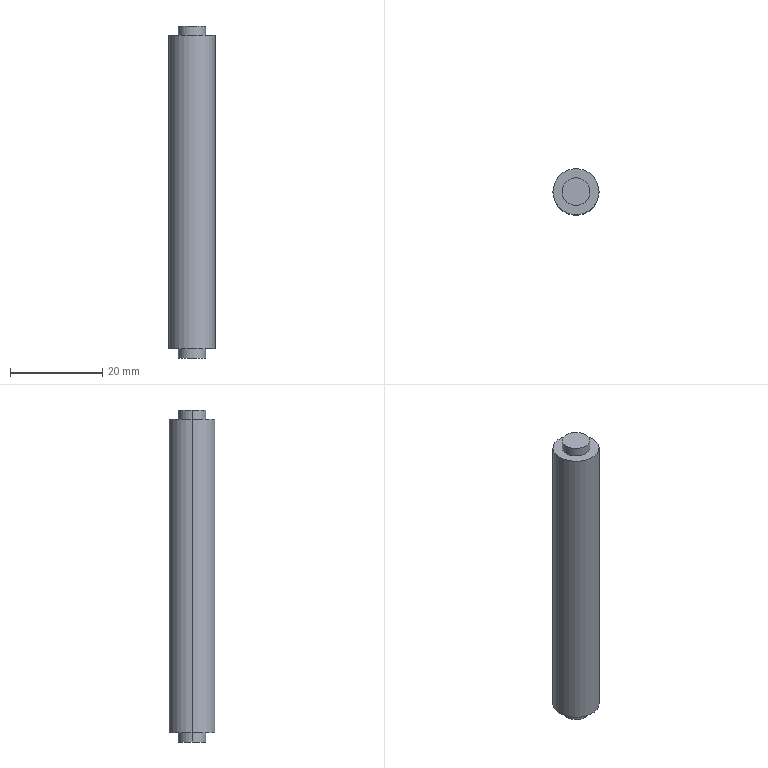Part | STEP file | 1 solid | 10 faces | box 10 x 10 x 72 mm | volume 5454 mm3 | cylinder 6 | plane 4 | commonest cylinder face diameters 6 x4 10 x2
STEP:
#1=CARTESIAN_POINT('',(0.,0.,0.));
#2=DIRECTION('',(0.,0.,1.));
#3=DIRECTION('',(1.,0.,0.));
#4=AXIS2_PLACEMENT_3D('',#1,#2,#3);
#5=CARTESIAN_POINT('',(182.13,-201.166,-34.));
#6=VERTEX_POINT('',#5);
#7=CARTESIAN_POINT('',(172.13,-201.166,-34.));
#8=VERTEX_POINT('',#7);
#9=CARTESIAN_POINT('',(177.13,-201.166,-34.));
#10=DIRECTION('',(0.,0.,1.));
#11=DIRECTION('',(1.,0.,0.));
#12=AXIS2_PLACEMENT_3D('',#9,#10,#11);
#13=CIRCLE('',#12,5.);
#14=CARTESIAN_POINT('',(177.13,-201.166,0.));
#15=DIRECTION('',(0.,0.,1.));
#16=DIRECTION('',(1.,0.,0.));
#17=AXIS2_PLACEMENT_3D('',#14,#15,#16);
#18=CYLINDRICAL_SURFACE('',#17,5.);
#19=CARTESIAN_POINT('',(0.,-34.));
#20=DIRECTION('',(1.,0.));
#21=VECTOR('',#20,1.);
#22=LINE('',#19,#21);
#23=(GEOMETRIC_REPRESENTATION_CONTEXT(2)PARAMETRIC_REPRESENTATION_CONTEXT()REPRESENTATION_CONTEXT('',''));
#24=DEFINITIONAL_REPRESENTATION('',(#22),#23);
#25=PCURVE('',#18,#24);
#26=CARTESIAN_POINT('',(177.13,-201.166,-34.));
#27=DIRECTION('',(0.,0.,1.));
#28=DIRECTION('',(1.,0.,0.));
#29=AXIS2_PLACEMENT_3D('',#26,#27,#28);
#30=PLANE('',#29);
#31=CARTESIAN_POINT('',(0.,0.));
#32=DIRECTION('',(1.,0.));
#33=AXIS2_PLACEMENT_2D('',#31,#32);
#34=CIRCLE('',#33,5.);
#35=(GEOMETRIC_REPRESENTATION_CONTEXT(2)PARAMETRIC_REPRESENTATION_CONTEXT()REPRESENTATION_CONTEXT('',''));
#36=DEFINITIONAL_REPRESENTATION('',(#34),#35);
#37=PCURVE('',#30,#36);
#38=SURFACE_CURVE('',#13,(#25,#37),.PCURVE_S1.);
#39=EDGE_CURVE('',#6,#8,#38,.T.);
#40=ORIENTED_EDGE('',*,*,#39,.T.);
#41=CARTESIAN_POINT('',(172.13,-201.166,34.));
#42=VERTEX_POINT('',#41);
#43=CARTESIAN_POINT('',(172.13,-201.166,0.));
#44=DIRECTION('',(0.,0.,1.));
#45=VECTOR('',#44,1.);
#46=LINE('',#43,#45);
#47=CARTESIAN_POINT('',(3.142,0.));
#48=DIRECTION('',(0.,1.));
#49=VECTOR('',#48,1.);
#50=LINE('',#47,#49);
#51=(GEOMETRIC_REPRESENTATION_CONTEXT(2)PARAMETRIC_REPRESENTATION_CONTEXT()REPRESENTATION_CONTEXT('',''));
#52=DEFINITIONAL_REPRESENTATION('',(#50),#51);
#53=PCURVE('',#18,#52);
#54=CARTESIAN_POINT('',(177.13,-201.166,0.));
#55=DIRECTION('',(0.,0.,1.));
#56=DIRECTION('',(1.,0.,0.));
#57=AXIS2_PLACEMENT_3D('',#54,#55,#56);
#58=CYLINDRICAL_SURFACE('',#57,5.);
#59=CARTESIAN_POINT('',(3.142,0.));
#60=DIRECTION('',(0.,1.));
#61=VECTOR('',#60,1.);
#62=LINE('',#59,#61);
#63=(GEOMETRIC_REPRESENTATION_CONTEXT(2)PARAMETRIC_REPRESENTATION_CONTEXT()REPRESENTATION_CONTEXT('',''));
#64=DEFINITIONAL_REPRESENTATION('',(#62),#63);
#65=PCURVE('',#58,#64);
#66=SURFACE_CURVE('',#46,(#53,#65),.PCURVE_S1.);
#67=EDGE_CURVE('',#8,#42,#66,.T.);
#68=ORIENTED_EDGE('',*,*,#67,.T.);
#69=CARTESIAN_POINT('',(182.13,-201.166,34.));
#70=VERTEX_POINT('',#69);
#71=CARTESIAN_POINT('',(177.13,-201.166,34.));
#72=DIRECTION('',(0.,0.,-1.));
#73=DIRECTION('',(1.,0.,0.));
#74=AXIS2_PLACEMENT_3D('',#71,#72,#73);
#75=CIRCLE('',#74,5.);
#76=CARTESIAN_POINT('',(6.283,34.));
#77=DIRECTION('',(-1.,0.));
#78=VECTOR('',#77,1.);
#79=LINE('',#76,#78);
#80=(GEOMETRIC_REPRESENTATION_CONTEXT(2)PARAMETRIC_REPRESENTATION_CONTEXT()REPRESENTATION_CONTEXT('',''));
#81=DEFINITIONAL_REPRESENTATION('',(#79),#80);
#82=PCURVE('',#18,#81);
#83=CARTESIAN_POINT('',(177.13,-201.166,34.));
#84=DIRECTION('',(0.,0.,1.));
#85=DIRECTION('',(1.,0.,0.));
#86=AXIS2_PLACEMENT_3D('',#83,#84,#85);
#87=PLANE('',#86);
#88=CARTESIAN_POINT('',(5.,0.));
#89=CARTESIAN_POINT('',(5.,-8.66));
#90=CARTESIAN_POINT('',(-2.5,-4.33));
#91=CARTESIAN_POINT('',(-10.,0.));
#92=CARTESIAN_POINT('',(-2.5,4.33));
#93=CARTESIAN_POINT('',(5.,8.66));
#94=CARTESIAN_POINT('',(5.,0.));
#95=(BOUNDED_CURVE()B_SPLINE_CURVE(2,(#88,#89,#90,#91,#92,#93,#94),.UNSPECIFIED.,.T.,.F.)B_SPLINE_CURVE_WITH_KNOTS((1,2,2,2,2,1),(-2.094,0.,2.094,4.189,6.283,8.378),.UNSPECIFIED.)CURVE()GEOMETRIC_REPRESENTATION_ITEM()RATIONAL_B_SPLINE_CURVE((1.,0.5,1.,0.5,1.,0.5,1.))REPRESENTATION_ITEM(''));
#96=(GEOMETRIC_REPRESENTATION_CONTEXT(2)PARAMETRIC_REPRESENTATION_CONTEXT()REPRESENTATION_CONTEXT('',''));
#97=DEFINITIONAL_REPRESENTATION('',(#95),#96);
#98=PCURVE('',#87,#97);
#99=SURFACE_CURVE('',#75,(#82,#98),.PCURVE_S1.);
#100=EDGE_CURVE('',#42,#70,#99,.T.);
#101=ORIENTED_EDGE('',*,*,#100,.T.);
#102=CARTESIAN_POINT('',(182.13,-201.166,0.));
#103=DIRECTION('',(0.,0.,1.));
#104=VECTOR('',#103,1.);
#105=LINE('',#102,#104);
#106=CARTESIAN_POINT('',(0.,0.));
#107=DIRECTION('',(0.,1.));
#108=VECTOR('',#107,1.);
#109=LINE('',#106,#108);
#110=(GEOMETRIC_REPRESENTATION_CONTEXT(2)PARAMETRIC_REPRESENTATION_CONTEXT()REPRESENTATION_CONTEXT('',''));
#111=DEFINITIONAL_REPRESENTATION('',(#109),#110);
#112=PCURVE('',#18,#111);
#113=CARTESIAN_POINT('',(6.283,0.));
#114=DIRECTION('',(0.,1.));
#115=VECTOR('',#114,1.);
#116=LINE('',#113,#115);
#117=(GEOMETRIC_REPRESENTATION_CONTEXT(2)PARAMETRIC_REPRESENTATION_CONTEXT()REPRESENTATION_CONTEXT('',''));
#118=DEFINITIONAL_REPRESENTATION('',(#116),#117);
#119=PCURVE('',#58,#118);
#120=SURFACE_CURVE('',#105,(#112,#119),.PCURVE_S1.);
#121=EDGE_CURVE('',#6,#70,#120,.T.);
#122=ORIENTED_EDGE('',*,*,#121,.F.);
#123=EDGE_LOOP('',(#40,#68,#101,#122));
#124=FACE_BOUND('',#123,.T.);
#125=ADVANCED_FACE('',(#124),#18,.T.);
#126=CARTESIAN_POINT('',(174.13,-201.166,36.));
#127=VERTEX_POINT('',#126);
#128=CARTESIAN_POINT('',(180.13,-201.166,36.));
#129=VERTEX_POINT('',#128);
#130=CARTESIAN_POINT('',(177.13,-201.166,36.));
#131=DIRECTION('',(0.,0.,-1.));
#132=DIRECTION('',(-1.,0.,0.));
#133=AXIS2_PLACEMENT_3D('',#130,#131,#132);
#134=CIRCLE('',#133,3.);
#135=CARTESIAN_POINT('',(177.13,-201.166,34.));
#136=DIRECTION('',(0.,0.,-1.));
#137=DIRECTION('',(-1.,0.,0.));
#138=AXIS2_PLACEMENT_3D('',#135,#136,#137);
#139=CYLINDRICAL_SURFACE('',#138,3.);
#140=CARTESIAN_POINT('',(0.,-2.));
#141=DIRECTION('',(1.,0.));
#142=VECTOR('',#141,1.);
#143=LINE('',#140,#142);
#144=(GEOMETRIC_REPRESENTATION_CONTEXT(2)PARAMETRIC_REPRESENTATION_CONTEXT()REPRESENTATION_CONTEXT('',''));
#145=DEFINITIONAL_REPRESENTATION('',(#143),#144);
#146=PCURVE('',#139,#145);
#147=CARTESIAN_POINT('',(177.13,-201.166,36.));
#148=DIRECTION('',(0.,0.,1.));
#149=DIRECTION('',(1.,0.,0.));
#150=AXIS2_PLACEMENT_3D('',#147,#148,#149);
#151=PLANE('',#150);
#152=CARTESIAN_POINT('',(-3.,0.));
#153=CARTESIAN_POINT('',(-3.,5.196));
#154=CARTESIAN_POINT('',(1.5,2.598));
#155=CARTESIAN_POINT('',(6.,0.));
#156=CARTESIAN_POINT('',(1.5,-2.598));
#157=CARTESIAN_POINT('',(-3.,-5.196));
#158=CARTESIAN_POINT('',(-3.,0.));
#159=(BOUNDED_CURVE()B_SPLINE_CURVE(2,(#152,#153,#154,#155,#156,#157,#158),.UNSPECIFIED.,.T.,.F.)B_SPLINE_CURVE_WITH_KNOTS((1,2,2,2,2,1),(-2.094,0.,2.094,4.189,6.283,8.378),.UNSPECIFIED.)CURVE()GEOMETRIC_REPRESENTATION_ITEM()RATIONAL_B_SPLINE_CURVE((1.,0.5,1.,0.5,1.,0.5,1.))REPRESENTATION_ITEM(''));
#160=(GEOMETRIC_REPRESENTATION_CONTEXT(2)PARAMETRIC_REPRESENTATION_CONTEXT()REPRESENTATION_CONTEXT('',''));
#161=DEFINITIONAL_REPRESENTATION('',(#159),#160);
#162=PCURVE('',#151,#161);
#163=SURFACE_CURVE('',#134,(#146,#162),.PCURVE_S1.);
#164=EDGE_CURVE('',#127,#129,#163,.T.);
#165=ORIENTED_EDGE('',*,*,#164,.T.);
#166=CARTESIAN_POINT('',(180.13,-201.166,34.));
#167=VERTEX_POINT('',#166);
#168=CARTESIAN_POINT('',(180.13,-201.166,34.));
#169=DIRECTION('',(0.,0.,-1.));
#170=VECTOR('',#169,1.);
#171=LINE('',#168,#170);
#172=CARTESIAN_POINT('',(3.142,0.));
#173=DIRECTION('',(0.,1.));
#174=VECTOR('',#173,1.);
#175=LINE('',#172,#174);
#176=(GEOMETRIC_REPRESENTATION_CONTEXT(2)PARAMETRIC_REPRESENTATION_CONTEXT()REPRESENTATION_CONTEXT('',''));
#177=DEFINITIONAL_REPRESENTATION('',(#175),#176);
#178=PCURVE('',#139,#177);
#179=CARTESIAN_POINT('',(177.13,-201.166,34.));
#180=DIRECTION('',(0.,0.,-1.));
#181=DIRECTION('',(-1.,0.,0.));
#182=AXIS2_PLACEMENT_3D('',#179,#180,#181);
#183=CYLINDRICAL_SURFACE('',#182,3.);
#184=CARTESIAN_POINT('',(3.142,0.));
#185=DIRECTION('',(0.,1.));
#186=VECTOR('',#185,1.);
#187=LINE('',#184,#186);
#188=(GEOMETRIC_REPRESENTATION_CONTEXT(2)PARAMETRIC_REPRESENTATION_CONTEXT()REPRESENTATION_CONTEXT('',''));
#189=DEFINITIONAL_REPRESENTATION('',(#187),#188);
#190=PCURVE('',#183,#189);
#191=SURFACE_CURVE('',#171,(#178,#190),.PCURVE_S1.);
#192=EDGE_CURVE('',#129,#167,#191,.T.);
#193=ORIENTED_EDGE('',*,*,#192,.T.);
#194=CARTESIAN_POINT('',(174.13,-201.166,34.));
#195=VERTEX_POINT('',#194);
#196=CARTESIAN_POINT('',(177.13,-201.166,34.));
#197=DIRECTION('',(0.,0.,-1.));
#198=DIRECTION('',(-1.,0.,0.));
#199=AXIS2_PLACEMENT_3D('',#196,#197,#198);
#200=CIRCLE('',#199,3.);
#201=CARTESIAN_POINT('',(0.,0.));
#202=DIRECTION('',(1.,0.));
#203=VECTOR('',#202,1.);
#204=LINE('',#201,#203);
#205=(GEOMETRIC_REPRESENTATION_CONTEXT(2)PARAMETRIC_REPRESENTATION_CONTEXT()REPRESENTATION_CONTEXT('',''));
#206=DEFINITIONAL_REPRESENTATION('',(#204),#205);
#207=PCURVE('',#139,#206);
#208=CARTESIAN_POINT('',(-3.,0.));
#209=CARTESIAN_POINT('',(-3.,5.196));
#210=CARTESIAN_POINT('',(1.5,2.598));
#211=CARTESIAN_POINT('',(6.,0.));
#212=CARTESIAN_POINT('',(1.5,-2.598));
#213=CARTESIAN_POINT('',(-3.,-5.196));
#214=CARTESIAN_POINT('',(-3.,0.));
#215=(BOUNDED_CURVE()B_SPLINE_CURVE(2,(#208,#209,#210,#211,#212,#213,#214),.UNSPECIFIED.,.T.,.F.)B_SPLINE_CURVE_WITH_KNOTS((1,2,2,2,2,1),(-2.094,0.,2.094,4.189,6.283,8.378),.UNSPECIFIED.)CURVE()GEOMETRIC_REPRESENTATION_ITEM()RATIONAL_B_SPLINE_CURVE((1.,0.5,1.,0.5,1.,0.5,1.))REPRESENTATION_ITEM(''));
#216=(GEOMETRIC_REPRESENTATION_CONTEXT(2)PARAMETRIC_REPRESENTATION_CONTEXT()REPRESENTATION_CONTEXT('',''));
#217=DEFINITIONAL_REPRESENTATION('',(#215),#216);
#218=PCURVE('',#87,#217);
#219=SURFACE_CURVE('',#200,(#207,#218),.PCURVE_S1.);
#220=EDGE_CURVE('',#195,#167,#219,.T.);
#221=ORIENTED_EDGE('',*,*,#220,.F.);
#222=CARTESIAN_POINT('',(174.13,-201.166,34.));
#223=DIRECTION('',(0.,0.,-1.));
#224=VECTOR('',#223,1.);
#225=LINE('',#222,#224);
#226=CARTESIAN_POINT('',(0.,0.));
#227=DIRECTION('',(0.,1.));
#228=VECTOR('',#227,1.);
#229=LINE('',#226,#228);
#230=(GEOMETRIC_REPRESENTATION_CONTEXT(2)PARAMETRIC_REPRESENTATION_CONTEXT()REPRESENTATION_CONTEXT('',''));
#231=DEFINITIONAL_REPRESENTATION('',(#229),#230);
#232=PCURVE('',#139,#231);
#233=CARTESIAN_POINT('',(6.283,0.));
#234=DIRECTION('',(0.,1.));
#235=VECTOR('',#234,1.);
#236=LINE('',#233,#235);
#237=(GEOMETRIC_REPRESENTATION_CONTEXT(2)PARAMETRIC_REPRESENTATION_CONTEXT()REPRESENTATION_CONTEXT('',''));
#238=DEFINITIONAL_REPRESENTATION('',(#236),#237);
#239=PCURVE('',#183,#238);
#240=SURFACE_CURVE('',#225,(#232,#239),.PCURVE_S1.);
#241=EDGE_CURVE('',#127,#195,#240,.T.);
#242=ORIENTED_EDGE('',*,*,#241,.F.);
#243=EDGE_LOOP('',(#165,#193,#221,#242));
#244=FACE_BOUND('',#243,.T.);
#245=ADVANCED_FACE('',(#244),#139,.T.);
#246=CARTESIAN_POINT('',(174.13,-201.166,-34.));
#247=VERTEX_POINT('',#246);
#248=CARTESIAN_POINT('',(180.13,-201.166,-34.));
#249=VERTEX_POINT('',#248);
#250=CARTESIAN_POINT('',(177.13,-201.166,-34.));
#251=DIRECTION('',(0.,0.,-1.));
#252=DIRECTION('',(-1.,0.,0.));
#253=AXIS2_PLACEMENT_3D('',#250,#251,#252);
#254=CIRCLE('',#253,3.);
#255=CARTESIAN_POINT('',(177.13,-201.166,-34.));
#256=DIRECTION('',(0.,0.,-1.));
#257=DIRECTION('',(-1.,0.,0.));
#258=AXIS2_PLACEMENT_3D('',#255,#256,#257);
#259=CYLINDRICAL_SURFACE('',#258,3.);
#260=CARTESIAN_POINT('',(0.,0.));
#261=DIRECTION('',(1.,0.));
#262=VECTOR('',#261,1.);
#263=LINE('',#260,#262);
#264=(GEOMETRIC_REPRESENTATION_CONTEXT(2)PARAMETRIC_REPRESENTATION_CONTEXT()REPRESENTATION_CONTEXT('',''));
#265=DEFINITIONAL_REPRESENTATION('',(#263),#264);
#266=PCURVE('',#259,#265);
#267=CARTESIAN_POINT('',(-3.,0.));
#268=CARTESIAN_POINT('',(-3.,5.196));
#269=CARTESIAN_POINT('',(1.5,2.598));
#270=CARTESIAN_POINT('',(6.,0.));
#271=CARTESIAN_POINT('',(1.5,-2.598));
#272=CARTESIAN_POINT('',(-3.,-5.196));
#273=CARTESIAN_POINT('',(-3.,0.));
#274=(BOUNDED_CURVE()B_SPLINE_CURVE(2,(#267,#268,#269,#270,#271,#272,#273),.UNSPECIFIED.,.T.,.F.)B_SPLINE_CURVE_WITH_KNOTS((1,2,2,2,2,1),(-2.094,0.,2.094,4.189,6.283,8.378),.UNSPECIFIED.)CURVE()GEOMETRIC_REPRESENTATION_ITEM()RATIONAL_B_SPLINE_CURVE((1.,0.5,1.,0.5,1.,0.5,1.))REPRESENTATION_ITEM(''));
#275=(GEOMETRIC_REPRESENTATION_CONTEXT(2)PARAMETRIC_REPRESENTATION_CONTEXT()REPRESENTATION_CONTEXT('',''));
#276=DEFINITIONAL_REPRESENTATION('',(#274),#275);
#277=PCURVE('',#30,#276);
#278=SURFACE_CURVE('',#254,(#266,#277),.PCURVE_S1.);
#279=EDGE_CURVE('',#247,#249,#278,.T.);
#280=ORIENTED_EDGE('',*,*,#279,.T.);
#281=CARTESIAN_POINT('',(180.13,-201.166,-36.));
#282=VERTEX_POINT('',#281);
#283=CARTESIAN_POINT('',(180.13,-201.166,-34.));
#284=DIRECTION('',(0.,0.,-1.));
#285=VECTOR('',#284,1.);
#286=LINE('',#283,#285);
#287=CARTESIAN_POINT('',(3.142,0.));
#288=DIRECTION('',(0.,1.));
#289=VECTOR('',#288,1.);
#290=LINE('',#287,#289);
#291=(GEOMETRIC_REPRESENTATION_CONTEXT(2)PARAMETRIC_REPRESENTATION_CONTEXT()REPRESENTATION_CONTEXT('',''));
#292=DEFINITIONAL_REPRESENTATION('',(#290),#291);
#293=PCURVE('',#259,#292);
#294=CARTESIAN_POINT('',(177.13,-201.166,-34.));
#295=DIRECTION('',(0.,0.,-1.));
#296=DIRECTION('',(-1.,0.,0.));
#297=AXIS2_PLACEMENT_3D('',#294,#295,#296);
#298=CYLINDRICAL_SURFACE('',#297,3.);
#299=CARTESIAN_POINT('',(3.142,0.));
#300=DIRECTION('',(0.,1.));
#301=VECTOR('',#300,1.);
#302=LINE('',#299,#301);
#303=(GEOMETRIC_REPRESENTATION_CONTEXT(2)PARAMETRIC_REPRESENTATION_CONTEXT()REPRESENTATION_CONTEXT('',''));
#304=DEFINITIONAL_REPRESENTATION('',(#302),#303);
#305=PCURVE('',#298,#304);
#306=SURFACE_CURVE('',#286,(#293,#305),.PCURVE_S1.);
#307=EDGE_CURVE('',#249,#282,#306,.T.);
#308=ORIENTED_EDGE('',*,*,#307,.T.);
#309=CARTESIAN_POINT('',(174.13,-201.166,-36.));
#310=VERTEX_POINT('',#309);
#311=CARTESIAN_POINT('',(177.13,-201.166,-36.));
#312=DIRECTION('',(0.,0.,1.));
#313=DIRECTION('',(-1.,0.,0.));
#314=AXIS2_PLACEMENT_3D('',#311,#312,#313);
#315=CIRCLE('',#314,3.);
#316=CARTESIAN_POINT('',(6.283,2.));
#317=DIRECTION('',(-1.,0.));
#318=VECTOR('',#317,1.);
#319=LINE('',#316,#318);
#320=(GEOMETRIC_REPRESENTATION_CONTEXT(2)PARAMETRIC_REPRESENTATION_CONTEXT()REPRESENTATION_CONTEXT('',''));
#321=DEFINITIONAL_REPRESENTATION('',(#319),#320);
#322=PCURVE('',#259,#321);
#323=CARTESIAN_POINT('',(177.13,-201.166,-36.));
#324=DIRECTION('',(0.,0.,1.));
#325=DIRECTION('',(1.,0.,0.));
#326=AXIS2_PLACEMENT_3D('',#323,#324,#325);
#327=PLANE('',#326);
#328=CARTESIAN_POINT('',(0.,0.));
#329=DIRECTION('',(-1.,0.));
#330=AXIS2_PLACEMENT_2D('',#328,#329);
#331=CIRCLE('',#330,3.);
#332=(GEOMETRIC_REPRESENTATION_CONTEXT(2)PARAMETRIC_REPRESENTATION_CONTEXT()REPRESENTATION_CONTEXT('',''));
#333=DEFINITIONAL_REPRESENTATION('',(#331),#332);
#334=PCURVE('',#327,#333);
#335=SURFACE_CURVE('',#315,(#322,#334),.PCURVE_S1.);
#336=EDGE_CURVE('',#282,#310,#335,.T.);
#337=ORIENTED_EDGE('',*,*,#336,.T.);
#338=CARTESIAN_POINT('',(174.13,-201.166,-34.));
#339=DIRECTION('',(0.,0.,-1.));
#340=VECTOR('',#339,1.);
#341=LINE('',#338,#340);
#342=CARTESIAN_POINT('',(0.,0.));
#343=DIRECTION('',(0.,1.));
#344=VECTOR('',#343,1.);
#345=LINE('',#342,#344);
#346=(GEOMETRIC_REPRESENTATION_CONTEXT(2)PARAMETRIC_REPRESENTATION_CONTEXT()REPRESENTATION_CONTEXT('',''));
#347=DEFINITIONAL_REPRESENTATION('',(#345),#346);
#348=PCURVE('',#259,#347);
#349=CARTESIAN_POINT('',(6.283,0.));
#350=DIRECTION('',(0.,1.));
#351=VECTOR('',#350,1.);
#352=LINE('',#349,#351);
#353=(GEOMETRIC_REPRESENTATION_CONTEXT(2)PARAMETRIC_REPRESENTATION_CONTEXT()REPRESENTATION_CONTEXT('',''));
#354=DEFINITIONAL_REPRESENTATION('',(#352),#353);
#355=PCURVE('',#298,#354);
#356=SURFACE_CURVE('',#341,(#348,#355),.PCURVE_S1.);
#357=EDGE_CURVE('',#247,#310,#356,.T.);
#358=ORIENTED_EDGE('',*,*,#357,.F.);
#359=EDGE_LOOP('',(#280,#308,#337,#358));
#360=FACE_BOUND('',#359,.T.);
#361=ADVANCED_FACE('',(#360),#259,.T.);
#362=ORIENTED_EDGE('',*,*,#67,.F.);
#363=CARTESIAN_POINT('',(177.13,-201.166,-34.));
#364=DIRECTION('',(0.,0.,1.));
#365=DIRECTION('',(1.,0.,0.));
#366=AXIS2_PLACEMENT_3D('',#363,#364,#365);
#367=CIRCLE('',#366,5.);
#368=CARTESIAN_POINT('',(0.,-34.));
#369=DIRECTION('',(1.,0.));
#370=VECTOR('',#369,1.);
#371=LINE('',#368,#370);
#372=(GEOMETRIC_REPRESENTATION_CONTEXT(2)PARAMETRIC_REPRESENTATION_CONTEXT()REPRESENTATION_CONTEXT('',''));
#373=DEFINITIONAL_REPRESENTATION('',(#371),#372);
#374=PCURVE('',#58,#373);
#375=CARTESIAN_POINT('',(0.,0.));
#376=DIRECTION('',(1.,0.));
#377=AXIS2_PLACEMENT_2D('',#375,#376);
#378=CIRCLE('',#377,5.);
#379=(GEOMETRIC_REPRESENTATION_CONTEXT(2)PARAMETRIC_REPRESENTATION_CONTEXT()REPRESENTATION_CONTEXT('',''));
#380=DEFINITIONAL_REPRESENTATION('',(#378),#379);
#381=PCURVE('',#30,#380);
#382=SURFACE_CURVE('',#367,(#374,#381),.PCURVE_S1.);
#383=EDGE_CURVE('',#8,#6,#382,.T.);
#384=ORIENTED_EDGE('',*,*,#383,.T.);
#385=ORIENTED_EDGE('',*,*,#121,.T.);
#386=CARTESIAN_POINT('',(177.13,-201.166,34.));
#387=DIRECTION('',(0.,0.,-1.));
#388=DIRECTION('',(1.,0.,0.));
#389=AXIS2_PLACEMENT_3D('',#386,#387,#388);
#390=CIRCLE('',#389,5.);
#391=CARTESIAN_POINT('',(6.283,34.));
#392=DIRECTION('',(-1.,0.));
#393=VECTOR('',#392,1.);
#394=LINE('',#391,#393);
#395=(GEOMETRIC_REPRESENTATION_CONTEXT(2)PARAMETRIC_REPRESENTATION_CONTEXT()REPRESENTATION_CONTEXT('',''));
#396=DEFINITIONAL_REPRESENTATION('',(#394),#395);
#397=PCURVE('',#58,#396);
#398=CARTESIAN_POINT('',(5.,0.));
#399=CARTESIAN_POINT('',(5.,-8.66));
#400=CARTESIAN_POINT('',(-2.5,-4.33));
#401=CARTESIAN_POINT('',(-10.,0.));
#402=CARTESIAN_POINT('',(-2.5,4.33));
#403=CARTESIAN_POINT('',(5.,8.66));
#404=CARTESIAN_POINT('',(5.,0.));
#405=(BOUNDED_CURVE()B_SPLINE_CURVE(2,(#398,#399,#400,#401,#402,#403,#404),.UNSPECIFIED.,.T.,.F.)B_SPLINE_CURVE_WITH_KNOTS((1,2,2,2,2,1),(-2.094,0.,2.094,4.189,6.283,8.378),.UNSPECIFIED.)CURVE()GEOMETRIC_REPRESENTATION_ITEM()RATIONAL_B_SPLINE_CURVE((1.,0.5,1.,0.5,1.,0.5,1.))REPRESENTATION_ITEM(''));
#406=(GEOMETRIC_REPRESENTATION_CONTEXT(2)PARAMETRIC_REPRESENTATION_CONTEXT()REPRESENTATION_CONTEXT('',''));
#407=DEFINITIONAL_REPRESENTATION('',(#405),#406);
#408=PCURVE('',#87,#407);
#409=SURFACE_CURVE('',#390,(#397,#408),.PCURVE_S1.);
#410=EDGE_CURVE('',#70,#42,#409,.T.);
#411=ORIENTED_EDGE('',*,*,#410,.T.);
#412=EDGE_LOOP('',(#362,#384,#385,#411));
#413=FACE_BOUND('',#412,.T.);
#414=ADVANCED_FACE('',(#413),#58,.T.);
#415=ORIENTED_EDGE('',*,*,#410,.F.);
#416=ORIENTED_EDGE('',*,*,#100,.F.);
#417=EDGE_LOOP('',(#415,#416));
#418=FACE_BOUND('',#417,.T.);
#419=ORIENTED_EDGE('',*,*,#220,.T.);
#420=CARTESIAN_POINT('',(177.13,-201.166,34.));
#421=DIRECTION('',(0.,0.,-1.));
#422=DIRECTION('',(-1.,0.,0.));
#423=AXIS2_PLACEMENT_3D('',#420,#421,#422);
#424=CIRCLE('',#423,3.);
#425=CARTESIAN_POINT('',(-3.,0.));
#426=CARTESIAN_POINT('',(-3.,5.196));
#427=CARTESIAN_POINT('',(1.5,2.598));
#428=CARTESIAN_POINT('',(6.,0.));
#429=CARTESIAN_POINT('',(1.5,-2.598));
#430=CARTESIAN_POINT('',(-3.,-5.196));
#431=CARTESIAN_POINT('',(-3.,0.));
#432=(BOUNDED_CURVE()B_SPLINE_CURVE(2,(#425,#426,#427,#428,#429,#430,#431),.UNSPECIFIED.,.T.,.F.)B_SPLINE_CURVE_WITH_KNOTS((1,2,2,2,2,1),(-2.094,0.,2.094,4.189,6.283,8.378),.UNSPECIFIED.)CURVE()GEOMETRIC_REPRESENTATION_ITEM()RATIONAL_B_SPLINE_CURVE((1.,0.5,1.,0.5,1.,0.5,1.))REPRESENTATION_ITEM(''));
#433=(GEOMETRIC_REPRESENTATION_CONTEXT(2)PARAMETRIC_REPRESENTATION_CONTEXT()REPRESENTATION_CONTEXT('',''));
#434=DEFINITIONAL_REPRESENTATION('',(#432),#433);
#435=PCURVE('',#87,#434);
#436=CARTESIAN_POINT('',(0.,0.));
#437=DIRECTION('',(1.,0.));
#438=VECTOR('',#437,1.);
#439=LINE('',#436,#438);
#440=(GEOMETRIC_REPRESENTATION_CONTEXT(2)PARAMETRIC_REPRESENTATION_CONTEXT()REPRESENTATION_CONTEXT('',''));
#441=DEFINITIONAL_REPRESENTATION('',(#439),#440);
#442=PCURVE('',#183,#441);
#443=SURFACE_CURVE('',#424,(#435,#442),.PCURVE_S1.);
#444=EDGE_CURVE('',#167,#195,#443,.T.);
#445=ORIENTED_EDGE('',*,*,#444,.T.);
#446=EDGE_LOOP('',(#419,#445));
#447=FACE_BOUND('',#446,.T.);
#448=ADVANCED_FACE('',(#418,#447),#87,.T.);
#449=ORIENTED_EDGE('',*,*,#39,.F.);
#450=ORIENTED_EDGE('',*,*,#383,.F.);
#451=EDGE_LOOP('',(#449,#450));
#452=FACE_BOUND('',#451,.T.);
#453=ORIENTED_EDGE('',*,*,#279,.F.);
#454=CARTESIAN_POINT('',(177.13,-201.166,-34.));
#455=DIRECTION('',(0.,0.,-1.));
#456=DIRECTION('',(-1.,0.,0.));
#457=AXIS2_PLACEMENT_3D('',#454,#455,#456);
#458=CIRCLE('',#457,3.);
#459=CARTESIAN_POINT('',(-3.,0.));
#460=CARTESIAN_POINT('',(-3.,5.196));
#461=CARTESIAN_POINT('',(1.5,2.598));
#462=CARTESIAN_POINT('',(6.,0.));
#463=CARTESIAN_POINT('',(1.5,-2.598));
#464=CARTESIAN_POINT('',(-3.,-5.196));
#465=CARTESIAN_POINT('',(-3.,0.));
#466=(BOUNDED_CURVE()B_SPLINE_CURVE(2,(#459,#460,#461,#462,#463,#464,#465),.UNSPECIFIED.,.T.,.F.)B_SPLINE_CURVE_WITH_KNOTS((1,2,2,2,2,1),(-2.094,0.,2.094,4.189,6.283,8.378),.UNSPECIFIED.)CURVE()GEOMETRIC_REPRESENTATION_ITEM()RATIONAL_B_SPLINE_CURVE((1.,0.5,1.,0.5,1.,0.5,1.))REPRESENTATION_ITEM(''));
#467=(GEOMETRIC_REPRESENTATION_CONTEXT(2)PARAMETRIC_REPRESENTATION_CONTEXT()REPRESENTATION_CONTEXT('',''));
#468=DEFINITIONAL_REPRESENTATION('',(#466),#467);
#469=PCURVE('',#30,#468);
#470=CARTESIAN_POINT('',(0.,0.));
#471=DIRECTION('',(1.,0.));
#472=VECTOR('',#471,1.);
#473=LINE('',#470,#472);
#474=(GEOMETRIC_REPRESENTATION_CONTEXT(2)PARAMETRIC_REPRESENTATION_CONTEXT()REPRESENTATION_CONTEXT('',''));
#475=DEFINITIONAL_REPRESENTATION('',(#473),#474);
#476=PCURVE('',#298,#475);
#477=SURFACE_CURVE('',#458,(#469,#476),.PCURVE_S1.);
#478=EDGE_CURVE('',#249,#247,#477,.T.);
#479=ORIENTED_EDGE('',*,*,#478,.F.);
#480=EDGE_LOOP('',(#453,#479));
#481=FACE_BOUND('',#480,.T.);
#482=ADVANCED_FACE('',(#452,#481),#30,.F.);
#483=ORIENTED_EDGE('',*,*,#192,.F.);
#484=CARTESIAN_POINT('',(177.13,-201.166,36.));
#485=DIRECTION('',(0.,0.,-1.));
#486=DIRECTION('',(-1.,0.,0.));
#487=AXIS2_PLACEMENT_3D('',#484,#485,#486);
#488=CIRCLE('',#487,3.);
#489=CARTESIAN_POINT('',(0.,-2.));
#490=DIRECTION('',(1.,0.));
#491=VECTOR('',#490,1.);
#492=LINE('',#489,#491);
#493=(GEOMETRIC_REPRESENTATION_CONTEXT(2)PARAMETRIC_REPRESENTATION_CONTEXT()REPRESENTATION_CONTEXT('',''));
#494=DEFINITIONAL_REPRESENTATION('',(#492),#493);
#495=PCURVE('',#183,#494);
#496=CARTESIAN_POINT('',(-3.,0.));
#497=CARTESIAN_POINT('',(-3.,5.196));
#498=CARTESIAN_POINT('',(1.5,2.598));
#499=CARTESIAN_POINT('',(6.,0.));
#500=CARTESIAN_POINT('',(1.5,-2.598));
#501=CARTESIAN_POINT('',(-3.,-5.196));
#502=CARTESIAN_POINT('',(-3.,0.));
#503=(BOUNDED_CURVE()B_SPLINE_CURVE(2,(#496,#497,#498,#499,#500,#501,#502),.UNSPECIFIED.,.T.,.F.)B_SPLINE_CURVE_WITH_KNOTS((1,2,2,2,2,1),(-2.094,0.,2.094,4.189,6.283,8.378),.UNSPECIFIED.)CURVE()GEOMETRIC_REPRESENTATION_ITEM()RATIONAL_B_SPLINE_CURVE((1.,0.5,1.,0.5,1.,0.5,1.))REPRESENTATION_ITEM(''));
#504=(GEOMETRIC_REPRESENTATION_CONTEXT(2)PARAMETRIC_REPRESENTATION_CONTEXT()REPRESENTATION_CONTEXT('',''));
#505=DEFINITIONAL_REPRESENTATION('',(#503),#504);
#506=PCURVE('',#151,#505);
#507=SURFACE_CURVE('',#488,(#495,#506),.PCURVE_S1.);
#508=EDGE_CURVE('',#129,#127,#507,.T.);
#509=ORIENTED_EDGE('',*,*,#508,.T.);
#510=ORIENTED_EDGE('',*,*,#241,.T.);
#511=ORIENTED_EDGE('',*,*,#444,.F.);
#512=EDGE_LOOP('',(#483,#509,#510,#511));
#513=FACE_BOUND('',#512,.T.);
#514=ADVANCED_FACE('',(#513),#183,.T.);
#515=ORIENTED_EDGE('',*,*,#307,.F.);
#516=ORIENTED_EDGE('',*,*,#478,.T.);
#517=ORIENTED_EDGE('',*,*,#357,.T.);
#518=CARTESIAN_POINT('',(177.13,-201.166,-36.));
#519=DIRECTION('',(0.,0.,1.));
#520=DIRECTION('',(-1.,0.,0.));
#521=AXIS2_PLACEMENT_3D('',#518,#519,#520);
#522=CIRCLE('',#521,3.);
#523=CARTESIAN_POINT('',(6.283,2.));
#524=DIRECTION('',(-1.,0.));
#525=VECTOR('',#524,1.);
#526=LINE('',#523,#525);
#527=(GEOMETRIC_REPRESENTATION_CONTEXT(2)PARAMETRIC_REPRESENTATION_CONTEXT()REPRESENTATION_CONTEXT('',''));
#528=DEFINITIONAL_REPRESENTATION('',(#526),#527);
#529=PCURVE('',#298,#528);
#530=CARTESIAN_POINT('',(0.,0.));
#531=DIRECTION('',(-1.,0.));
#532=AXIS2_PLACEMENT_2D('',#530,#531);
#533=CIRCLE('',#532,3.);
#534=(GEOMETRIC_REPRESENTATION_CONTEXT(2)PARAMETRIC_REPRESENTATION_CONTEXT()REPRESENTATION_CONTEXT('',''));
#535=DEFINITIONAL_REPRESENTATION('',(#533),#534);
#536=PCURVE('',#327,#535);
#537=SURFACE_CURVE('',#522,(#529,#536),.PCURVE_S1.);
#538=EDGE_CURVE('',#310,#282,#537,.T.);
#539=ORIENTED_EDGE('',*,*,#538,.T.);
#540=EDGE_LOOP('',(#515,#516,#517,#539));
#541=FACE_BOUND('',#540,.T.);
#542=ADVANCED_FACE('',(#541),#298,.T.);
#543=ORIENTED_EDGE('',*,*,#164,.F.);
#544=ORIENTED_EDGE('',*,*,#508,.F.);
#545=EDGE_LOOP('',(#543,#544));
#546=FACE_BOUND('',#545,.T.);
#547=ADVANCED_FACE('',(#546),#151,.T.);
#548=ORIENTED_EDGE('',*,*,#538,.F.);
#549=ORIENTED_EDGE('',*,*,#336,.F.);
#550=EDGE_LOOP('',(#548,#549));
#551=FACE_BOUND('',#550,.T.);
#552=ADVANCED_FACE('',(#551),#327,.F.);
#553=CLOSED_SHELL('',(#125,#245,#361,#414,#448,#482,#514,#542,#547,#552));
#554=MANIFOLD_SOLID_BREP('',#553);
#555=(LENGTH_UNIT()NAMED_UNIT(*)SI_UNIT(.MILLI.,.METRE.));
#556=UNCERTAINTY_MEASURE_WITH_UNIT(LENGTH_MEASURE(0.0000001),#555,'','');
#557=(NAMED_UNIT(*)PLANE_ANGLE_UNIT()SI_UNIT($,.RADIAN.));
#558=(NAMED_UNIT(*)SI_UNIT($,.STERADIAN.)SOLID_ANGLE_UNIT());
#559=(GEOMETRIC_REPRESENTATION_CONTEXT(3)GLOBAL_UNCERTAINTY_ASSIGNED_CONTEXT((#556))GLOBAL_UNIT_ASSIGNED_CONTEXT((#555,#557,#558))REPRESENTATION_CONTEXT('',''));
#560=ADVANCED_BREP_SHAPE_REPRESENTATION('',(#4,#554),#559);